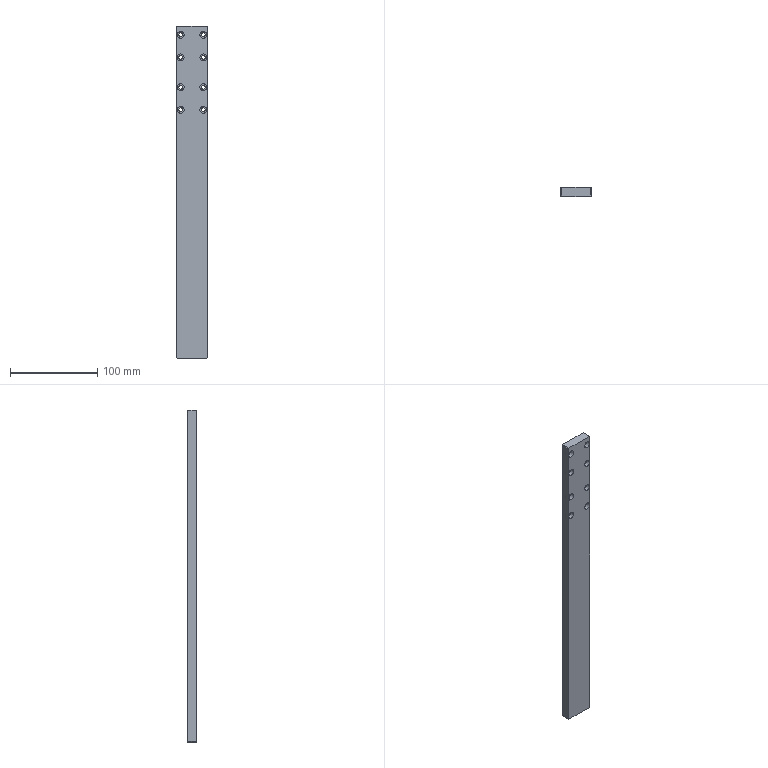Part | SolidWorks | features BaseBody 1 | 1 solid | 62 faces | box 35 x 10 x 380 mm | volume 129960 mm3 | cylinder 38 | plane 18 | cone 6 | commonest cylinder face diameters 4.5 x16 8 x16 3.3 x4 5 x2